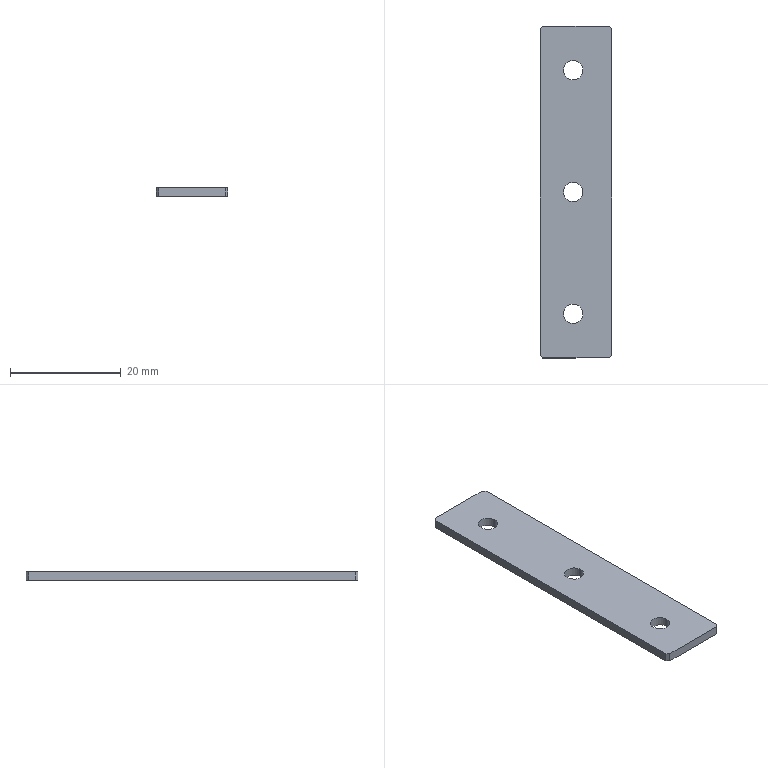Part | STEP file | Second Door Spacer PN_0025 Default | 1 solid | 16 faces | box 13 x 60 x 1.6 mm | volume 1201 mm3 | plane 10 | cylinder 6 | commonest cylinder face diameters 3.5 x6
STEP:
#1=CARTESIAN_POINT('',(-2.25,22.,0.));
#2=VERTEX_POINT('',#1);
#3=CARTESIAN_POINT('',(1.25,22.,0.));
#4=VERTEX_POINT('',#3);
#5=CARTESIAN_POINT('',(-0.5,22.,0.));
#6=DIRECTION('',(0.,0.,1.));
#7=DIRECTION('',(1.,0.,0.));
#8=AXIS2_PLACEMENT_3D('',#5,#6,#7);
#9=CIRCLE('',#8,1.75);
#10=EDGE_CURVE('',#2,#4,#9,.T.);
#11=ORIENTED_EDGE('',*,*,#10,.F.);
#12=CARTESIAN_POINT('',(-2.25,22.,1.6));
#13=VERTEX_POINT('',#12);
#14=CARTESIAN_POINT('',(-2.25,22.,1.6));
#15=DIRECTION('',(0.,0.,1.));
#16=VECTOR('',#15,1000.);
#17=LINE('',#14,#16);
#18=EDGE_CURVE('',#2,#13,#17,.T.);
#19=ORIENTED_EDGE('',*,*,#18,.T.);
#20=CARTESIAN_POINT('',(1.25,22.,1.6));
#21=VERTEX_POINT('',#20);
#22=CARTESIAN_POINT('',(-0.5,22.,1.6));
#23=DIRECTION('',(0.,0.,1.));
#24=DIRECTION('',(1.,0.,0.));
#25=AXIS2_PLACEMENT_3D('',#22,#23,#24);
#26=CIRCLE('',#25,1.75);
#27=EDGE_CURVE('',#13,#21,#26,.T.);
#28=ORIENTED_EDGE('',*,*,#27,.T.);
#29=CARTESIAN_POINT('',(1.25,22.,1.6));
#30=DIRECTION('',(0.,0.,1.));
#31=VECTOR('',#30,1000.);
#32=LINE('',#29,#31);
#33=EDGE_CURVE('',#4,#21,#32,.T.);
#34=ORIENTED_EDGE('',*,*,#33,.F.);
#35=EDGE_LOOP('',(#11,#19,#28,#34));
#36=FACE_OUTER_BOUND('',#35,.T.);
#37=CARTESIAN_POINT('',(-0.5,22.,1.6));
#38=DIRECTION('',(0.,0.,1.));
#39=DIRECTION('',(1.,0.,0.));
#40=AXIS2_PLACEMENT_3D('',#37,#38,#39);
#41=CYLINDRICAL_SURFACE('',#40,1.75);
#42=ADVANCED_FACE('',(#36),#41,.F.);
#43=CARTESIAN_POINT('',(-2.25,0.,0.));
#44=VERTEX_POINT('',#43);
#45=CARTESIAN_POINT('',(1.25,0.,0.));
#46=VERTEX_POINT('',#45);
#47=CARTESIAN_POINT('',(-0.5,0.,0.));
#48=DIRECTION('',(0.,0.,1.));
#49=DIRECTION('',(1.,0.,0.));
#50=AXIS2_PLACEMENT_3D('',#47,#48,#49);
#51=CIRCLE('',#50,1.75);
#52=EDGE_CURVE('',#44,#46,#51,.T.);
#53=ORIENTED_EDGE('',*,*,#52,.F.);
#54=CARTESIAN_POINT('',(-2.25,0.,1.6));
#55=VERTEX_POINT('',#54);
#56=CARTESIAN_POINT('',(-2.25,0.,1.6));
#57=DIRECTION('',(0.,0.,1.));
#58=VECTOR('',#57,1000.);
#59=LINE('',#56,#58);
#60=EDGE_CURVE('',#44,#55,#59,.T.);
#61=ORIENTED_EDGE('',*,*,#60,.T.);
#62=CARTESIAN_POINT('',(1.25,0.,1.6));
#63=VERTEX_POINT('',#62);
#64=CARTESIAN_POINT('',(-0.5,0.,1.6));
#65=DIRECTION('',(0.,0.,1.));
#66=DIRECTION('',(1.,0.,0.));
#67=AXIS2_PLACEMENT_3D('',#64,#65,#66);
#68=CIRCLE('',#67,1.75);
#69=EDGE_CURVE('',#55,#63,#68,.T.);
#70=ORIENTED_EDGE('',*,*,#69,.T.);
#71=CARTESIAN_POINT('',(1.25,0.,1.6));
#72=DIRECTION('',(0.,0.,1.));
#73=VECTOR('',#72,1000.);
#74=LINE('',#71,#73);
#75=EDGE_CURVE('',#46,#63,#74,.T.);
#76=ORIENTED_EDGE('',*,*,#75,.F.);
#77=EDGE_LOOP('',(#53,#61,#70,#76));
#78=FACE_OUTER_BOUND('',#77,.T.);
#79=CARTESIAN_POINT('',(-0.5,0.,1.6));
#80=DIRECTION('',(0.,0.,1.));
#81=DIRECTION('',(1.,0.,0.));
#82=AXIS2_PLACEMENT_3D('',#79,#80,#81);
#83=CYLINDRICAL_SURFACE('',#82,1.75);
#84=ADVANCED_FACE('',(#78),#83,.F.);
#85=CARTESIAN_POINT('',(-2.25,-22.,0.));
#86=VERTEX_POINT('',#85);
#87=CARTESIAN_POINT('',(1.25,-22.,0.));
#88=VERTEX_POINT('',#87);
#89=CARTESIAN_POINT('',(-0.5,-22.,0.));
#90=DIRECTION('',(0.,0.,1.));
#91=DIRECTION('',(1.,0.,0.));
#92=AXIS2_PLACEMENT_3D('',#89,#90,#91);
#93=CIRCLE('',#92,1.75);
#94=EDGE_CURVE('',#86,#88,#93,.T.);
#95=ORIENTED_EDGE('',*,*,#94,.F.);
#96=CARTESIAN_POINT('',(-2.25,-22.,1.6));
#97=VERTEX_POINT('',#96);
#98=CARTESIAN_POINT('',(-2.25,-22.,1.6));
#99=DIRECTION('',(0.,0.,1.));
#100=VECTOR('',#99,1000.);
#101=LINE('',#98,#100);
#102=EDGE_CURVE('',#86,#97,#101,.T.);
#103=ORIENTED_EDGE('',*,*,#102,.T.);
#104=CARTESIAN_POINT('',(1.25,-22.,1.6));
#105=VERTEX_POINT('',#104);
#106=CARTESIAN_POINT('',(-0.5,-22.,1.6));
#107=DIRECTION('',(0.,0.,1.));
#108=DIRECTION('',(1.,0.,0.));
#109=AXIS2_PLACEMENT_3D('',#106,#107,#108);
#110=CIRCLE('',#109,1.75);
#111=EDGE_CURVE('',#97,#105,#110,.T.);
#112=ORIENTED_EDGE('',*,*,#111,.T.);
#113=CARTESIAN_POINT('',(1.25,-22.,1.6));
#114=DIRECTION('',(0.,0.,1.));
#115=VECTOR('',#114,1000.);
#116=LINE('',#113,#115);
#117=EDGE_CURVE('',#88,#105,#116,.T.);
#118=ORIENTED_EDGE('',*,*,#117,.F.);
#119=EDGE_LOOP('',(#95,#103,#112,#118));
#120=FACE_OUTER_BOUND('',#119,.T.);
#121=CARTESIAN_POINT('',(-0.5,-22.,1.6));
#122=DIRECTION('',(0.,0.,1.));
#123=DIRECTION('',(1.,0.,0.));
#124=AXIS2_PLACEMENT_3D('',#121,#122,#123);
#125=CYLINDRICAL_SURFACE('',#124,1.75);
#126=ADVANCED_FACE('',(#120),#125,.F.);
#127=CARTESIAN_POINT('',(-6.5,29.5,1.6));
#128=VERTEX_POINT('',#127);
#129=CARTESIAN_POINT('',(-6.5,-29.5,1.6));
#130=VERTEX_POINT('',#129);
#131=CARTESIAN_POINT('',(-6.5,-30.,1.6));
#132=DIRECTION('',(0.,-1.,0.));
#133=VECTOR('',#132,1000.);
#134=LINE('',#131,#133);
#135=EDGE_CURVE('',#128,#130,#134,.T.);
#136=ORIENTED_EDGE('',*,*,#135,.F.);
#137=CARTESIAN_POINT('',(-6.5,29.5,0.));
#138=VERTEX_POINT('',#137);
#139=CARTESIAN_POINT('',(-6.5,29.5,1.6));
#140=DIRECTION('',(0.,0.,-1.));
#141=VECTOR('',#140,1000.);
#142=LINE('',#139,#141);
#143=EDGE_CURVE('',#128,#138,#142,.T.);
#144=ORIENTED_EDGE('',*,*,#143,.T.);
#145=CARTESIAN_POINT('',(-6.5,-29.5,0.));
#146=VERTEX_POINT('',#145);
#147=CARTESIAN_POINT('',(-6.5,-30.,0.));
#148=DIRECTION('',(0.,-1.,0.));
#149=VECTOR('',#148,1000.);
#150=LINE('',#147,#149);
#151=EDGE_CURVE('',#138,#146,#150,.T.);
#152=ORIENTED_EDGE('',*,*,#151,.T.);
#153=CARTESIAN_POINT('',(-6.5,-29.5,1.6));
#154=DIRECTION('',(0.,0.,1.));
#155=VECTOR('',#154,1000.);
#156=LINE('',#153,#155);
#157=EDGE_CURVE('',#146,#130,#156,.T.);
#158=ORIENTED_EDGE('',*,*,#157,.T.);
#159=EDGE_LOOP('',(#136,#144,#152,#158));
#160=FACE_OUTER_BOUND('',#159,.T.);
#161=CARTESIAN_POINT('',(-6.5,-30.,1.6));
#162=DIRECTION('',(1.,0.,0.));
#163=DIRECTION('',(0.,0.,-1.));
#164=AXIS2_PLACEMENT_3D('',#161,#162,#163);
#165=PLANE('',#164);
#166=ADVANCED_FACE('',(#160),#165,.F.);
#167=CARTESIAN_POINT('',(-6.,-30.,0.));
#168=VERTEX_POINT('',#167);
#169=CARTESIAN_POINT('',(6.,-30.,0.));
#170=VERTEX_POINT('',#169);
#171=CARTESIAN_POINT('',(6.5,-30.,0.));
#172=DIRECTION('',(1.,0.,0.));
#173=VECTOR('',#172,1000.);
#174=LINE('',#171,#173);
#175=EDGE_CURVE('',#168,#170,#174,.T.);
#176=ORIENTED_EDGE('',*,*,#175,.T.);
#177=CARTESIAN_POINT('',(6.,-30.,1.6));
#178=VERTEX_POINT('',#177);
#179=CARTESIAN_POINT('',(6.,-30.,1.6));
#180=DIRECTION('',(0.,0.,1.));
#181=VECTOR('',#180,1000.);
#182=LINE('',#179,#181);
#183=EDGE_CURVE('',#170,#178,#182,.T.);
#184=ORIENTED_EDGE('',*,*,#183,.T.);
#185=CARTESIAN_POINT('',(-6.,-30.,1.6));
#186=VERTEX_POINT('',#185);
#187=CARTESIAN_POINT('',(6.5,-30.,1.6));
#188=DIRECTION('',(1.,0.,0.));
#189=VECTOR('',#188,1000.);
#190=LINE('',#187,#189);
#191=EDGE_CURVE('',#186,#178,#190,.T.);
#192=ORIENTED_EDGE('',*,*,#191,.F.);
#193=CARTESIAN_POINT('',(-6.,-30.,1.6));
#194=DIRECTION('',(0.,0.,-1.));
#195=VECTOR('',#194,1000.);
#196=LINE('',#193,#195);
#197=EDGE_CURVE('',#186,#168,#196,.T.);
#198=ORIENTED_EDGE('',*,*,#197,.T.);
#199=EDGE_LOOP('',(#176,#184,#192,#198));
#200=FACE_OUTER_BOUND('',#199,.T.);
#201=CARTESIAN_POINT('',(6.5,-30.,1.6));
#202=DIRECTION('',(0.,1.,0.));
#203=DIRECTION('',(-1.,0.,0.));
#204=AXIS2_PLACEMENT_3D('',#201,#202,#203);
#205=PLANE('',#204);
#206=ADVANCED_FACE('',(#200),#205,.F.);
#207=CARTESIAN_POINT('',(6.5,-29.5,0.));
#208=VERTEX_POINT('',#207);
#209=CARTESIAN_POINT('',(6.5,29.5,0.));
#210=VERTEX_POINT('',#209);
#211=CARTESIAN_POINT('',(6.5,-30.,0.));
#212=DIRECTION('',(0.,1.,0.));
#213=VECTOR('',#212,1000.);
#214=LINE('',#211,#213);
#215=EDGE_CURVE('',#208,#210,#214,.T.);
#216=ORIENTED_EDGE('',*,*,#215,.T.);
#217=CARTESIAN_POINT('',(6.5,29.5,1.6));
#218=VERTEX_POINT('',#217);
#219=CARTESIAN_POINT('',(6.5,29.5,1.6));
#220=DIRECTION('',(0.,0.,1.));
#221=VECTOR('',#220,1000.);
#222=LINE('',#219,#221);
#223=EDGE_CURVE('',#210,#218,#222,.T.);
#224=ORIENTED_EDGE('',*,*,#223,.T.);
#225=CARTESIAN_POINT('',(6.5,-29.5,1.6));
#226=VERTEX_POINT('',#225);
#227=CARTESIAN_POINT('',(6.5,-30.,1.6));
#228=DIRECTION('',(0.,1.,0.));
#229=VECTOR('',#228,1000.);
#230=LINE('',#227,#229);
#231=EDGE_CURVE('',#226,#218,#230,.T.);
#232=ORIENTED_EDGE('',*,*,#231,.F.);
#233=CARTESIAN_POINT('',(6.5,-29.5,1.6));
#234=DIRECTION('',(0.,0.,-1.));
#235=VECTOR('',#234,1000.);
#236=LINE('',#233,#235);
#237=EDGE_CURVE('',#226,#208,#236,.T.);
#238=ORIENTED_EDGE('',*,*,#237,.T.);
#239=EDGE_LOOP('',(#216,#224,#232,#238));
#240=FACE_OUTER_BOUND('',#239,.T.);
#241=CARTESIAN_POINT('',(6.5,-30.,1.6));
#242=DIRECTION('',(-1.,0.,0.));
#243=DIRECTION('',(0.,0.,1.));
#244=AXIS2_PLACEMENT_3D('',#241,#242,#243);
#245=PLANE('',#244);
#246=ADVANCED_FACE('',(#240),#245,.F.);
#247=CARTESIAN_POINT('',(6.,30.,0.));
#248=VERTEX_POINT('',#247);
#249=CARTESIAN_POINT('',(-6.,30.,0.));
#250=VERTEX_POINT('',#249);
#251=CARTESIAN_POINT('',(6.5,30.,0.));
#252=DIRECTION('',(-1.,0.,0.));
#253=VECTOR('',#252,1000.);
#254=LINE('',#251,#253);
#255=EDGE_CURVE('',#248,#250,#254,.T.);
#256=ORIENTED_EDGE('',*,*,#255,.T.);
#257=CARTESIAN_POINT('',(-6.,30.,1.6));
#258=VERTEX_POINT('',#257);
#259=CARTESIAN_POINT('',(-6.,30.,1.6));
#260=DIRECTION('',(0.,0.,1.));
#261=VECTOR('',#260,1000.);
#262=LINE('',#259,#261);
#263=EDGE_CURVE('',#250,#258,#262,.T.);
#264=ORIENTED_EDGE('',*,*,#263,.T.);
#265=CARTESIAN_POINT('',(6.,30.,1.6));
#266=VERTEX_POINT('',#265);
#267=CARTESIAN_POINT('',(6.5,30.,1.6));
#268=DIRECTION('',(-1.,0.,0.));
#269=VECTOR('',#268,1000.);
#270=LINE('',#267,#269);
#271=EDGE_CURVE('',#266,#258,#270,.T.);
#272=ORIENTED_EDGE('',*,*,#271,.F.);
#273=CARTESIAN_POINT('',(6.,30.,1.6));
#274=DIRECTION('',(0.,0.,-1.));
#275=VECTOR('',#274,1000.);
#276=LINE('',#273,#275);
#277=EDGE_CURVE('',#266,#248,#276,.T.);
#278=ORIENTED_EDGE('',*,*,#277,.T.);
#279=EDGE_LOOP('',(#256,#264,#272,#278));
#280=FACE_OUTER_BOUND('',#279,.T.);
#281=CARTESIAN_POINT('',(6.5,30.,1.6));
#282=DIRECTION('',(0.,-1.,0.));
#283=DIRECTION('',(0.,0.,-1.));
#284=AXIS2_PLACEMENT_3D('',#281,#282,#283);
#285=PLANE('',#284);
#286=ADVANCED_FACE('',(#280),#285,.F.);
#287=CARTESIAN_POINT('',(-0.5,22.,1.6));
#288=DIRECTION('',(0.,0.,1.));
#289=DIRECTION('',(1.,0.,0.));
#290=AXIS2_PLACEMENT_3D('',#287,#288,#289);
#291=CIRCLE('',#290,1.75);
#292=EDGE_CURVE('',#21,#13,#291,.T.);
#293=ORIENTED_EDGE('',*,*,#292,.F.);
#294=ORIENTED_EDGE('',*,*,#27,.F.);
#295=EDGE_LOOP('',(#293,#294));
#296=FACE_BOUND('',#295,.T.);
#297=CARTESIAN_POINT('',(-0.5,0.,1.6));
#298=DIRECTION('',(0.,0.,1.));
#299=DIRECTION('',(1.,0.,0.));
#300=AXIS2_PLACEMENT_3D('',#297,#298,#299);
#301=CIRCLE('',#300,1.75);
#302=EDGE_CURVE('',#63,#55,#301,.T.);
#303=ORIENTED_EDGE('',*,*,#302,.F.);
#304=ORIENTED_EDGE('',*,*,#69,.F.);
#305=EDGE_LOOP('',(#303,#304));
#306=FACE_BOUND('',#305,.T.);
#307=CARTESIAN_POINT('',(-0.5,-22.,1.6));
#308=DIRECTION('',(0.,0.,1.));
#309=DIRECTION('',(1.,0.,0.));
#310=AXIS2_PLACEMENT_3D('',#307,#308,#309);
#311=CIRCLE('',#310,1.75);
#312=EDGE_CURVE('',#105,#97,#311,.T.);
#313=ORIENTED_EDGE('',*,*,#312,.F.);
#314=ORIENTED_EDGE('',*,*,#111,.F.);
#315=EDGE_LOOP('',(#313,#314));
#316=FACE_BOUND('',#315,.T.);
#317=ORIENTED_EDGE('',*,*,#271,.T.);
#318=CARTESIAN_POINT('',(-18.,18.,1.6));
#319=DIRECTION('',(-0.7071,-0.7071,0.));
#320=VECTOR('',#319,1000.);
#321=LINE('',#318,#320);
#322=EDGE_CURVE('',#258,#128,#321,.T.);
#323=ORIENTED_EDGE('',*,*,#322,.T.);
#324=ORIENTED_EDGE('',*,*,#135,.T.);
#325=CARTESIAN_POINT('',(-18.,-18.,1.6));
#326=DIRECTION('',(0.7071,-0.7071,0.));
#327=VECTOR('',#326,1000.);
#328=LINE('',#325,#327);
#329=EDGE_CURVE('',#130,#186,#328,.T.);
#330=ORIENTED_EDGE('',*,*,#329,.T.);
#331=ORIENTED_EDGE('',*,*,#191,.T.);
#332=CARTESIAN_POINT('',(18.,-18.,1.6));
#333=DIRECTION('',(0.7071,0.7071,0.));
#334=VECTOR('',#333,1000.);
#335=LINE('',#332,#334);
#336=EDGE_CURVE('',#178,#226,#335,.T.);
#337=ORIENTED_EDGE('',*,*,#336,.T.);
#338=ORIENTED_EDGE('',*,*,#231,.T.);
#339=CARTESIAN_POINT('',(18.,18.,1.6));
#340=DIRECTION('',(-0.7071,0.7071,0.));
#341=VECTOR('',#340,1000.);
#342=LINE('',#339,#341);
#343=EDGE_CURVE('',#218,#266,#342,.T.);
#344=ORIENTED_EDGE('',*,*,#343,.T.);
#345=EDGE_LOOP('',(#317,#323,#324,#330,#331,#337,#338,#344));
#346=FACE_OUTER_BOUND('',#345,.T.);
#347=CARTESIAN_POINT('',(0.,0.,1.6));
#348=DIRECTION('',(0.,0.,1.));
#349=DIRECTION('',(1.,0.,0.));
#350=AXIS2_PLACEMENT_3D('',#347,#348,#349);
#351=PLANE('',#350);
#352=ADVANCED_FACE('',(#296,#306,#316,#346),#351,.T.);
#353=CARTESIAN_POINT('',(-0.5,22.,0.));
#354=DIRECTION('',(0.,0.,1.));
#355=DIRECTION('',(1.,0.,0.));
#356=AXIS2_PLACEMENT_3D('',#353,#354,#355);
#357=CIRCLE('',#356,1.75);
#358=EDGE_CURVE('',#4,#2,#357,.T.);
#359=ORIENTED_EDGE('',*,*,#358,.T.);
#360=ORIENTED_EDGE('',*,*,#10,.T.);
#361=EDGE_LOOP('',(#359,#360));
#362=FACE_BOUND('',#361,.T.);
#363=CARTESIAN_POINT('',(-0.5,0.,0.));
#364=DIRECTION('',(0.,0.,1.));
#365=DIRECTION('',(1.,0.,0.));
#366=AXIS2_PLACEMENT_3D('',#363,#364,#365);
#367=CIRCLE('',#366,1.75);
#368=EDGE_CURVE('',#46,#44,#367,.T.);
#369=ORIENTED_EDGE('',*,*,#368,.T.);
#370=ORIENTED_EDGE('',*,*,#52,.T.);
#371=EDGE_LOOP('',(#369,#370));
#372=FACE_BOUND('',#371,.T.);
#373=CARTESIAN_POINT('',(-0.5,-22.,0.));
#374=DIRECTION('',(0.,0.,1.));
#375=DIRECTION('',(1.,0.,0.));
#376=AXIS2_PLACEMENT_3D('',#373,#374,#375);
#377=CIRCLE('',#376,1.75);
#378=EDGE_CURVE('',#88,#86,#377,.T.);
#379=ORIENTED_EDGE('',*,*,#378,.T.);
#380=ORIENTED_EDGE('',*,*,#94,.T.);
#381=EDGE_LOOP('',(#379,#380));
#382=FACE_BOUND('',#381,.T.);
#383=ORIENTED_EDGE('',*,*,#151,.F.);
#384=CARTESIAN_POINT('',(-6.5,29.5,0.));
#385=DIRECTION('',(0.7071,0.7071,0.));
#386=VECTOR('',#385,1000.);
#387=LINE('',#384,#386);
#388=EDGE_CURVE('',#138,#250,#387,.T.);
#389=ORIENTED_EDGE('',*,*,#388,.T.);
#390=ORIENTED_EDGE('',*,*,#255,.F.);
#391=CARTESIAN_POINT('',(6.,30.,0.));
#392=DIRECTION('',(0.7071,-0.7071,0.));
#393=VECTOR('',#392,1000.);
#394=LINE('',#391,#393);
#395=EDGE_CURVE('',#248,#210,#394,.T.);
#396=ORIENTED_EDGE('',*,*,#395,.T.);
#397=ORIENTED_EDGE('',*,*,#215,.F.);
#398=CARTESIAN_POINT('',(6.5,-29.5,0.));
#399=DIRECTION('',(-0.7071,-0.7071,0.));
#400=VECTOR('',#399,1000.);
#401=LINE('',#398,#400);
#402=EDGE_CURVE('',#208,#170,#401,.T.);
#403=ORIENTED_EDGE('',*,*,#402,.T.);
#404=ORIENTED_EDGE('',*,*,#175,.F.);
#405=CARTESIAN_POINT('',(-6.,-30.,0.));
#406=DIRECTION('',(-0.7071,0.7071,0.));
#407=VECTOR('',#406,1000.);
#408=LINE('',#405,#407);
#409=EDGE_CURVE('',#168,#146,#408,.T.);
#410=ORIENTED_EDGE('',*,*,#409,.T.);
#411=EDGE_LOOP('',(#383,#389,#390,#396,#397,#403,#404,#410));
#412=FACE_OUTER_BOUND('',#411,.T.);
#413=CARTESIAN_POINT('',(0.,0.,0.));
#414=DIRECTION('',(0.,0.,1.));
#415=DIRECTION('',(1.,0.,0.));
#416=AXIS2_PLACEMENT_3D('',#413,#414,#415);
#417=PLANE('',#416);
#418=ADVANCED_FACE('',(#362,#372,#382,#412),#417,.F.);
#419=ORIENTED_EDGE('',*,*,#102,.F.);
#420=ORIENTED_EDGE('',*,*,#378,.F.);
#421=ORIENTED_EDGE('',*,*,#117,.T.);
#422=ORIENTED_EDGE('',*,*,#312,.T.);
#423=EDGE_LOOP('',(#419,#420,#421,#422));
#424=FACE_OUTER_BOUND('',#423,.T.);
#425=CARTESIAN_POINT('',(-0.5,-22.,1.6));
#426=DIRECTION('',(0.,0.,1.));
#427=DIRECTION('',(1.,0.,0.));
#428=AXIS2_PLACEMENT_3D('',#425,#426,#427);
#429=CYLINDRICAL_SURFACE('',#428,1.75);
#430=ADVANCED_FACE('',(#424),#429,.F.);
#431=ORIENTED_EDGE('',*,*,#60,.F.);
#432=ORIENTED_EDGE('',*,*,#368,.F.);
#433=ORIENTED_EDGE('',*,*,#75,.T.);
#434=ORIENTED_EDGE('',*,*,#302,.T.);
#435=EDGE_LOOP('',(#431,#432,#433,#434));
#436=FACE_OUTER_BOUND('',#435,.T.);
#437=CARTESIAN_POINT('',(-0.5,0.,1.6));
#438=DIRECTION('',(0.,0.,1.));
#439=DIRECTION('',(1.,0.,0.));
#440=AXIS2_PLACEMENT_3D('',#437,#438,#439);
#441=CYLINDRICAL_SURFACE('',#440,1.75);
#442=ADVANCED_FACE('',(#436),#441,.F.);
#443=ORIENTED_EDGE('',*,*,#18,.F.);
#444=ORIENTED_EDGE('',*,*,#358,.F.);
#445=ORIENTED_EDGE('',*,*,#33,.T.);
#446=ORIENTED_EDGE('',*,*,#292,.T.);
#447=EDGE_LOOP('',(#443,#444,#445,#446));
#448=FACE_OUTER_BOUND('',#447,.T.);
#449=CARTESIAN_POINT('',(-0.5,22.,1.6));
#450=DIRECTION('',(0.,0.,1.));
#451=DIRECTION('',(1.,0.,0.));
#452=AXIS2_PLACEMENT_3D('',#449,#450,#451);
#453=CYLINDRICAL_SURFACE('',#452,1.75);
#454=ADVANCED_FACE('',(#448),#453,.F.);
#455=ORIENTED_EDGE('',*,*,#322,.F.);
#456=ORIENTED_EDGE('',*,*,#263,.F.);
#457=ORIENTED_EDGE('',*,*,#388,.F.);
#458=ORIENTED_EDGE('',*,*,#143,.F.);
#459=EDGE_LOOP('',(#455,#456,#457,#458));
#460=FACE_OUTER_BOUND('',#459,.T.);
#461=CARTESIAN_POINT('',(-6.5,29.5,1.6));
#462=DIRECTION('',(0.7071,-0.7071,0.));
#463=DIRECTION('',(0.,0.,-1.));
#464=AXIS2_PLACEMENT_3D('',#461,#462,#463);
#465=PLANE('',#464);
#466=ADVANCED_FACE('',(#460),#465,.F.);
#467=ORIENTED_EDGE('',*,*,#343,.F.);
#468=ORIENTED_EDGE('',*,*,#223,.F.);
#469=ORIENTED_EDGE('',*,*,#395,.F.);
#470=ORIENTED_EDGE('',*,*,#277,.F.);
#471=EDGE_LOOP('',(#467,#468,#469,#470));
#472=FACE_OUTER_BOUND('',#471,.T.);
#473=CARTESIAN_POINT('',(6.,30.,1.6));
#474=DIRECTION('',(-0.7071,-0.7071,0.));
#475=DIRECTION('',(0.,0.,-1.));
#476=AXIS2_PLACEMENT_3D('',#473,#474,#475);
#477=PLANE('',#476);
#478=ADVANCED_FACE('',(#472),#477,.F.);
#479=ORIENTED_EDGE('',*,*,#336,.F.);
#480=ORIENTED_EDGE('',*,*,#183,.F.);
#481=ORIENTED_EDGE('',*,*,#402,.F.);
#482=ORIENTED_EDGE('',*,*,#237,.F.);
#483=EDGE_LOOP('',(#479,#480,#481,#482));
#484=FACE_OUTER_BOUND('',#483,.T.);
#485=CARTESIAN_POINT('',(6.5,-29.5,1.6));
#486=DIRECTION('',(-0.7071,0.7071,0.));
#487=DIRECTION('',(0.,0.,-1.));
#488=AXIS2_PLACEMENT_3D('',#485,#486,#487);
#489=PLANE('',#488);
#490=ADVANCED_FACE('',(#484),#489,.F.);
#491=ORIENTED_EDGE('',*,*,#329,.F.);
#492=ORIENTED_EDGE('',*,*,#157,.F.);
#493=ORIENTED_EDGE('',*,*,#409,.F.);
#494=ORIENTED_EDGE('',*,*,#197,.F.);
#495=EDGE_LOOP('',(#491,#492,#493,#494));
#496=FACE_OUTER_BOUND('',#495,.T.);
#497=CARTESIAN_POINT('',(-6.,-30.,1.6));
#498=DIRECTION('',(0.7071,0.7071,0.));
#499=DIRECTION('',(0.,0.,-1.));
#500=AXIS2_PLACEMENT_3D('',#497,#498,#499);
#501=PLANE('',#500);
#502=ADVANCED_FACE('',(#496),#501,.F.);
#503=CLOSED_SHELL('',(#42,#84,#126,#166,#206,#246,#286,#352,#418,#430,#442,#454,#466,#478,#490,#502));
#504=MANIFOLD_SOLID_BREP('',#503);
#505=CARTESIAN_POINT('',(0.,0.,0.));
#506=DIRECTION('',(0.,0.,1.));
#507=DIRECTION('',(1.,0.,0.));
#508=AXIS2_PLACEMENT_3D('',#505,#506,#507);
#509=(LENGTH_UNIT()NAMED_UNIT(*)SI_UNIT(.MILLI.,.METRE.));
#510=UNCERTAINTY_MEASURE_WITH_UNIT(LENGTH_MEASURE(0.00001),#509,'','');
#511=(NAMED_UNIT(*)PLANE_ANGLE_UNIT()SI_UNIT($,.RADIAN.));
#512=(NAMED_UNIT(*)SI_UNIT($,.STERADIAN.)SOLID_ANGLE_UNIT());
#513=(GEOMETRIC_REPRESENTATION_CONTEXT(3)GLOBAL_UNCERTAINTY_ASSIGNED_CONTEXT((#510))GLOBAL_UNIT_ASSIGNED_CONTEXT((#509,#511,#512))REPRESENTATION_CONTEXT('',''));
#514=ADVANCED_BREP_SHAPE_REPRESENTATION('',(#504,#508),#513);